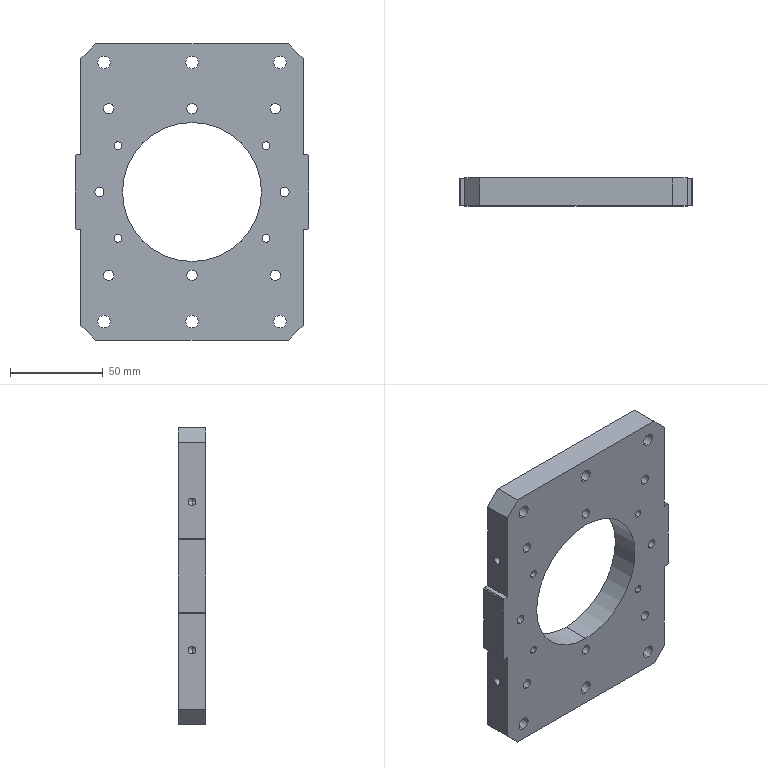Part | SolidWorks | features Cut 5, ICE 4, 3DProfileFeature 3, HoleWzd 3, Chamfer 2, Extrusion 1, MirrorPattern 1 | 1 solid | 100 faces | box 126 x 15 x 160 mm | volume 213891 mm3 | cylinder 62 | plane 30 | cone 8 | commonest cylinder face diameters 4.2 x16 5.5 x12 6.8 x12 12 x12 5 x4 8 x4